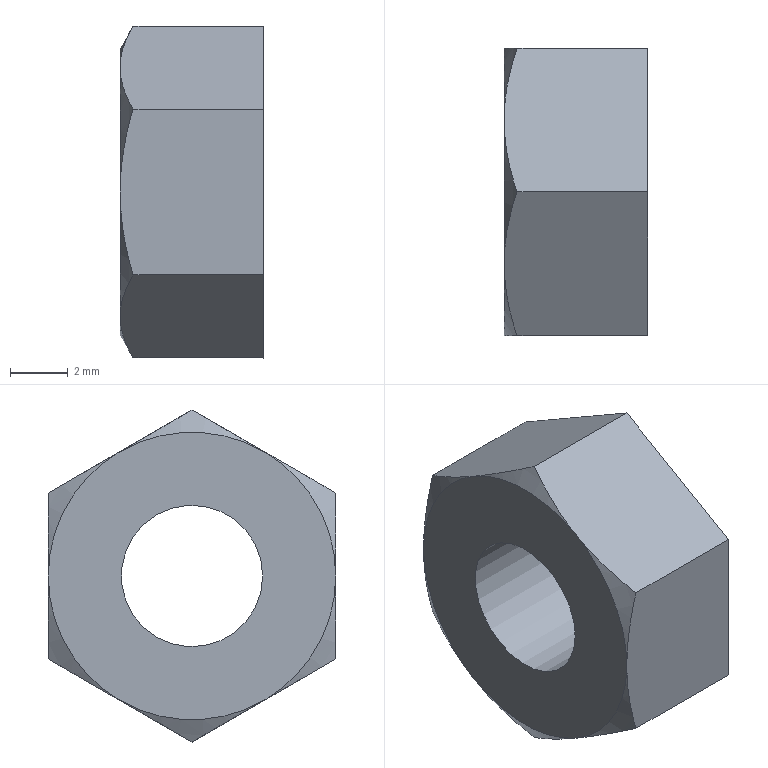Part | NX | features 5003_316_SLBNR6 2 | 1 solid | 15 faces | box 5 x 10 x 11.547 mm | volume 336.962 mm3 | plane 8 | cone 6 | cylinder 1 | commonest cylinder face diameters 4.917 x1
STEP:
#1=CARTESIAN_POINT('',(13.972,-167.,-217.113));
#2=VERTEX_POINT('',#1);
#3=CARTESIAN_POINT('',(18.525,-167.,-217.113));
#4=VERTEX_POINT('',#3);
#5=CARTESIAN_POINT('',(13.525,-167.,-217.113));
#6=DIRECTION('',(1.,0.,0.));
#7=VECTOR('',#6,1000.);
#8=LINE('',#5,#7);
#9=EDGE_CURVE('',#2,#4,#8,.T.);
#10=ORIENTED_EDGE('',*,*,#9,.F.);
#11=CARTESIAN_POINT('',(13.525,-169.5,-215.67));
#12=VERTEX_POINT('',#11);
#13=CARTESIAN_POINT('',(13.972,-167.,-217.113));
#14=CARTESIAN_POINT('',(13.699,-167.818,-216.641));
#15=CARTESIAN_POINT('',(13.525,-168.648,-216.162));
#16=CARTESIAN_POINT('',(13.525,-169.5,-215.67));
#17=B_SPLINE_CURVE_WITH_KNOTS('',3,(#13,#14,#15,#16),.UNSPECIFIED.,.F.,.F.,(4,4),(0.000000238,0.002921),.UNSPECIFIED.);
#18=EDGE_CURVE('',#2,#12,#17,.T.);
#19=ORIENTED_EDGE('',*,*,#18,.T.);
#20=CARTESIAN_POINT('',(13.972,-172.,-214.226));
#21=VERTEX_POINT('',#20);
#22=CARTESIAN_POINT('',(13.525,-169.5,-215.67));
#23=CARTESIAN_POINT('',(13.525,-170.349,-215.18));
#24=CARTESIAN_POINT('',(13.7,-171.184,-214.698));
#25=CARTESIAN_POINT('',(13.972,-172.,-214.226));
#26=B_SPLINE_CURVE_WITH_KNOTS('',3,(#22,#23,#24,#25),.UNSPECIFIED.,.F.,.F.,(4,4),(0.002921,0.005831),.UNSPECIFIED.);
#27=EDGE_CURVE('',#12,#21,#26,.T.);
#28=ORIENTED_EDGE('',*,*,#27,.T.);
#29=CARTESIAN_POINT('',(18.525,-172.,-214.226));
#30=VERTEX_POINT('',#29);
#31=CARTESIAN_POINT('',(13.525,-172.,-214.226));
#32=DIRECTION('',(1.,0.,0.));
#33=VECTOR('',#32,1000.);
#34=LINE('',#31,#33);
#35=EDGE_CURVE('',#21,#30,#34,.T.);
#36=ORIENTED_EDGE('',*,*,#35,.T.);
#37=CARTESIAN_POINT('',(18.525,-167.,-217.113));
#38=DIRECTION('',(0.,-0.866,0.5));
#39=VECTOR('',#38,1000.);
#40=LINE('',#37,#39);
#41=EDGE_CURVE('',#4,#30,#40,.T.);
#42=ORIENTED_EDGE('',*,*,#41,.F.);
#43=EDGE_LOOP('',(#10,#19,#28,#36,#42));
#44=FACE_BOUND('',#43,.T.);
#45=CARTESIAN_POINT('',(13.525,-167.,-217.113));
#46=DIRECTION('',(0.,0.5,0.866));
#47=DIRECTION('',(0.,-0.866,0.5));
#48=AXIS2_PLACEMENT_3D('',#45,#46,#47);
#49=PLANE('',#48);
#50=ADVANCED_FACE('',(#44),#49,.T.);
#51=CARTESIAN_POINT('',(13.972,-167.,-222.887));
#52=VERTEX_POINT('',#51);
#53=CARTESIAN_POINT('',(18.525,-167.,-222.887));
#54=VERTEX_POINT('',#53);
#55=CARTESIAN_POINT('',(13.525,-167.,-222.887));
#56=DIRECTION('',(1.,0.,0.));
#57=VECTOR('',#56,1000.);
#58=LINE('',#55,#57);
#59=EDGE_CURVE('',#52,#54,#58,.T.);
#60=ORIENTED_EDGE('',*,*,#59,.F.);
#61=CARTESIAN_POINT('',(13.525,-167.,-220.));
#62=VERTEX_POINT('',#61);
#63=CARTESIAN_POINT('',(13.972,-167.,-222.887));
#64=CARTESIAN_POINT('',(13.701,-167.,-221.948));
#65=CARTESIAN_POINT('',(13.525,-167.,-220.976));
#66=CARTESIAN_POINT('',(13.525,-167.,-220.));
#67=B_SPLINE_CURVE_WITH_KNOTS('',3,(#63,#64,#65,#66),.UNSPECIFIED.,.F.,.F.,(4,4),(0.00515,0.008071),.UNSPECIFIED.);
#68=EDGE_CURVE('',#52,#62,#67,.T.);
#69=ORIENTED_EDGE('',*,*,#68,.T.);
#70=CARTESIAN_POINT('',(13.525,-167.,-220.));
#71=CARTESIAN_POINT('',(13.525,-167.,-219.024));
#72=CARTESIAN_POINT('',(13.702,-167.,-218.047));
#73=CARTESIAN_POINT('',(13.972,-167.,-217.113));
#74=B_SPLINE_CURVE_WITH_KNOTS('',3,(#70,#71,#72,#73),.UNSPECIFIED.,.F.,.F.,(4,4),(0.008071,0.01099),.UNSPECIFIED.);
#75=EDGE_CURVE('',#62,#2,#74,.T.);
#76=ORIENTED_EDGE('',*,*,#75,.T.);
#77=ORIENTED_EDGE('',*,*,#9,.T.);
#78=CARTESIAN_POINT('',(18.525,-167.,-222.887));
#79=DIRECTION('',(0.,0.,1.));
#80=VECTOR('',#79,1000.);
#81=LINE('',#78,#80);
#82=EDGE_CURVE('',#54,#4,#81,.T.);
#83=ORIENTED_EDGE('',*,*,#82,.F.);
#84=EDGE_LOOP('',(#60,#69,#76,#77,#83));
#85=FACE_BOUND('',#84,.T.);
#86=CARTESIAN_POINT('',(13.525,-167.,-222.887));
#87=DIRECTION('',(0.,1.,0.));
#88=DIRECTION('',(0.,0.,1.));
#89=AXIS2_PLACEMENT_3D('',#86,#87,#88);
#90=PLANE('',#89);
#91=ADVANCED_FACE('',(#85),#90,.T.);
#92=CARTESIAN_POINT('',(13.972,-172.,-225.774));
#93=VERTEX_POINT('',#92);
#94=CARTESIAN_POINT('',(18.525,-172.,-225.774));
#95=VERTEX_POINT('',#94);
#96=CARTESIAN_POINT('',(13.525,-172.,-225.774));
#97=DIRECTION('',(1.,0.,0.));
#98=VECTOR('',#97,1000.);
#99=LINE('',#96,#98);
#100=EDGE_CURVE('',#93,#95,#99,.T.);
#101=ORIENTED_EDGE('',*,*,#100,.F.);
#102=CARTESIAN_POINT('',(13.525,-169.5,-224.33));
#103=VERTEX_POINT('',#102);
#104=CARTESIAN_POINT('',(13.972,-172.,-225.774));
#105=CARTESIAN_POINT('',(13.699,-171.182,-225.301));
#106=CARTESIAN_POINT('',(13.525,-170.352,-224.822));
#107=CARTESIAN_POINT('',(13.525,-169.5,-224.33));
#108=B_SPLINE_CURVE_WITH_KNOTS('',3,(#104,#105,#106,#107),.UNSPECIFIED.,.F.,.F.,(4,4),(0.000000238,0.002921),.UNSPECIFIED.);
#109=EDGE_CURVE('',#93,#103,#108,.T.);
#110=ORIENTED_EDGE('',*,*,#109,.T.);
#111=CARTESIAN_POINT('',(13.525,-169.5,-224.33));
#112=CARTESIAN_POINT('',(13.525,-168.651,-223.84));
#113=CARTESIAN_POINT('',(13.7,-167.816,-223.358));
#114=CARTESIAN_POINT('',(13.972,-167.,-222.887));
#115=B_SPLINE_CURVE_WITH_KNOTS('',3,(#111,#112,#113,#114),.UNSPECIFIED.,.F.,.F.,(4,4),(0.002921,0.005831),.UNSPECIFIED.);
#116=EDGE_CURVE('',#103,#52,#115,.T.);
#117=ORIENTED_EDGE('',*,*,#116,.T.);
#118=ORIENTED_EDGE('',*,*,#59,.T.);
#119=CARTESIAN_POINT('',(18.525,-172.,-225.774));
#120=DIRECTION('',(0.,0.866,0.5));
#121=VECTOR('',#120,1000.);
#122=LINE('',#119,#121);
#123=EDGE_CURVE('',#95,#54,#122,.T.);
#124=ORIENTED_EDGE('',*,*,#123,.F.);
#125=EDGE_LOOP('',(#101,#110,#117,#118,#124));
#126=FACE_BOUND('',#125,.T.);
#127=CARTESIAN_POINT('',(13.525,-172.,-225.774));
#128=DIRECTION('',(0.,0.5,-0.866));
#129=DIRECTION('',(0.,0.866,0.5));
#130=AXIS2_PLACEMENT_3D('',#127,#128,#129);
#131=PLANE('',#130);
#132=ADVANCED_FACE('',(#126),#131,.T.);
#133=CARTESIAN_POINT('',(13.972,-177.,-222.887));
#134=VERTEX_POINT('',#133);
#135=CARTESIAN_POINT('',(18.525,-177.,-222.887));
#136=VERTEX_POINT('',#135);
#137=CARTESIAN_POINT('',(13.525,-177.,-222.887));
#138=DIRECTION('',(1.,0.,0.));
#139=VECTOR('',#138,1000.);
#140=LINE('',#137,#139);
#141=EDGE_CURVE('',#134,#136,#140,.T.);
#142=ORIENTED_EDGE('',*,*,#141,.F.);
#143=CARTESIAN_POINT('',(13.525,-174.5,-224.33));
#144=VERTEX_POINT('',#143);
#145=CARTESIAN_POINT('',(13.972,-177.,-222.887));
#146=CARTESIAN_POINT('',(13.699,-176.182,-223.359));
#147=CARTESIAN_POINT('',(13.525,-175.352,-223.838));
#148=CARTESIAN_POINT('',(13.525,-174.5,-224.33));
#149=B_SPLINE_CURVE_WITH_KNOTS('',3,(#145,#146,#147,#148),.UNSPECIFIED.,.F.,.F.,(4,4),(0.000000238,0.002921),.UNSPECIFIED.);
#150=EDGE_CURVE('',#134,#144,#149,.T.);
#151=ORIENTED_EDGE('',*,*,#150,.T.);
#152=CARTESIAN_POINT('',(13.525,-174.5,-224.33));
#153=CARTESIAN_POINT('',(13.525,-173.651,-224.82));
#154=CARTESIAN_POINT('',(13.7,-172.816,-225.302));
#155=CARTESIAN_POINT('',(13.972,-172.,-225.774));
#156=B_SPLINE_CURVE_WITH_KNOTS('',3,(#152,#153,#154,#155),.UNSPECIFIED.,.F.,.F.,(4,4),(0.002921,0.005831),.UNSPECIFIED.);
#157=EDGE_CURVE('',#144,#93,#156,.T.);
#158=ORIENTED_EDGE('',*,*,#157,.T.);
#159=ORIENTED_EDGE('',*,*,#100,.T.);
#160=CARTESIAN_POINT('',(18.525,-177.,-222.887));
#161=DIRECTION('',(0.,0.866,-0.5));
#162=VECTOR('',#161,1000.);
#163=LINE('',#160,#162);
#164=EDGE_CURVE('',#136,#95,#163,.T.);
#165=ORIENTED_EDGE('',*,*,#164,.F.);
#166=EDGE_LOOP('',(#142,#151,#158,#159,#165));
#167=FACE_BOUND('',#166,.T.);
#168=CARTESIAN_POINT('',(13.525,-177.,-222.887));
#169=DIRECTION('',(0.,-0.5,-0.866));
#170=DIRECTION('',(0.,0.866,-0.5));
#171=AXIS2_PLACEMENT_3D('',#168,#169,#170);
#172=PLANE('',#171);
#173=ADVANCED_FACE('',(#167),#172,.T.);
#174=CARTESIAN_POINT('',(13.972,-177.,-217.113));
#175=VERTEX_POINT('',#174);
#176=CARTESIAN_POINT('',(18.525,-177.,-217.113));
#177=VERTEX_POINT('',#176);
#178=CARTESIAN_POINT('',(13.525,-177.,-217.113));
#179=DIRECTION('',(1.,0.,0.));
#180=VECTOR('',#179,1000.);
#181=LINE('',#178,#180);
#182=EDGE_CURVE('',#175,#177,#181,.T.);
#183=ORIENTED_EDGE('',*,*,#182,.F.);
#184=CARTESIAN_POINT('',(13.525,-177.,-220.));
#185=VERTEX_POINT('',#184);
#186=CARTESIAN_POINT('',(13.525,-177.,-220.));
#187=CARTESIAN_POINT('',(13.525,-177.,-219.024));
#188=CARTESIAN_POINT('',(13.702,-177.,-218.047));
#189=CARTESIAN_POINT('',(13.972,-177.,-217.113));
#190=B_SPLINE_CURVE_WITH_KNOTS('',3,(#186,#187,#188,#189),.UNSPECIFIED.,.F.,.F.,(4,4),(0.008071,0.01099),.UNSPECIFIED.);
#191=EDGE_CURVE('',#175,#185,#190,.F.);
#192=ORIENTED_EDGE('',*,*,#191,.T.);
#193=CARTESIAN_POINT('',(13.972,-177.,-222.887));
#194=CARTESIAN_POINT('',(13.701,-177.,-221.948));
#195=CARTESIAN_POINT('',(13.525,-177.,-220.976));
#196=CARTESIAN_POINT('',(13.525,-177.,-220.));
#197=B_SPLINE_CURVE_WITH_KNOTS('',3,(#193,#194,#195,#196),.UNSPECIFIED.,.F.,.F.,(4,4),(0.00515,0.008071),.UNSPECIFIED.);
#198=EDGE_CURVE('',#185,#134,#197,.F.);
#199=ORIENTED_EDGE('',*,*,#198,.T.);
#200=ORIENTED_EDGE('',*,*,#141,.T.);
#201=CARTESIAN_POINT('',(18.525,-177.,-217.113));
#202=DIRECTION('',(0.,0.,-1.));
#203=VECTOR('',#202,1000.);
#204=LINE('',#201,#203);
#205=EDGE_CURVE('',#177,#136,#204,.T.);
#206=ORIENTED_EDGE('',*,*,#205,.F.);
#207=EDGE_LOOP('',(#183,#192,#199,#200,#206));
#208=FACE_BOUND('',#207,.T.);
#209=CARTESIAN_POINT('',(13.525,-177.,-217.113));
#210=DIRECTION('',(0.,-1.,0.));
#211=DIRECTION('',(0.,0.,-1.));
#212=AXIS2_PLACEMENT_3D('',#209,#210,#211);
#213=PLANE('',#212);
#214=ADVANCED_FACE('',(#208),#213,.T.);
#215=ORIENTED_EDGE('',*,*,#35,.F.);
#216=CARTESIAN_POINT('',(13.525,-174.5,-215.67));
#217=VERTEX_POINT('',#216);
#218=CARTESIAN_POINT('',(13.972,-172.,-214.226));
#219=CARTESIAN_POINT('',(13.699,-172.818,-214.699));
#220=CARTESIAN_POINT('',(13.525,-173.648,-215.178));
#221=CARTESIAN_POINT('',(13.525,-174.5,-215.67));
#222=B_SPLINE_CURVE_WITH_KNOTS('',3,(#218,#219,#220,#221),.UNSPECIFIED.,.F.,.F.,(4,4),(0.000000238,0.002921),.UNSPECIFIED.);
#223=EDGE_CURVE('',#21,#217,#222,.T.);
#224=ORIENTED_EDGE('',*,*,#223,.T.);
#225=CARTESIAN_POINT('',(13.525,-174.5,-215.67));
#226=CARTESIAN_POINT('',(13.525,-175.349,-216.16));
#227=CARTESIAN_POINT('',(13.7,-176.184,-216.642));
#228=CARTESIAN_POINT('',(13.972,-177.,-217.113));
#229=B_SPLINE_CURVE_WITH_KNOTS('',3,(#225,#226,#227,#228),.UNSPECIFIED.,.F.,.F.,(4,4),(0.002921,0.005831),.UNSPECIFIED.);
#230=EDGE_CURVE('',#217,#175,#229,.T.);
#231=ORIENTED_EDGE('',*,*,#230,.T.);
#232=ORIENTED_EDGE('',*,*,#182,.T.);
#233=CARTESIAN_POINT('',(18.525,-172.,-214.226));
#234=DIRECTION('',(0.,-0.866,-0.5));
#235=VECTOR('',#234,1000.);
#236=LINE('',#233,#235);
#237=EDGE_CURVE('',#30,#177,#236,.T.);
#238=ORIENTED_EDGE('',*,*,#237,.F.);
#239=EDGE_LOOP('',(#215,#224,#231,#232,#238));
#240=FACE_BOUND('',#239,.T.);
#241=CARTESIAN_POINT('',(13.525,-172.,-214.226));
#242=DIRECTION('',(0.,-0.5,0.866));
#243=DIRECTION('',(0.,-0.866,-0.5));
#244=AXIS2_PLACEMENT_3D('',#241,#242,#243);
#245=PLANE('',#244);
#246=ADVANCED_FACE('',(#240),#245,.T.);
#247=CARTESIAN_POINT('',(18.525,-174.458,-220.));
#248=VERTEX_POINT('',#247);
#249=CARTESIAN_POINT('',(18.525,-172.,-220.));
#250=DIRECTION('',(-1.,0.,0.));
#251=DIRECTION('',(0.,-1.,0.));
#252=AXIS2_PLACEMENT_3D('',#249,#250,#251);
#253=CIRCLE('',#252,2.458);
#254=EDGE_CURVE('',#248,#248,#253,.T.);
#255=ORIENTED_EDGE('',*,*,#254,.T.);
#256=EDGE_LOOP('',(#255));
#257=FACE_BOUND('',#256,.T.);
#258=ORIENTED_EDGE('',*,*,#41,.T.);
#259=ORIENTED_EDGE('',*,*,#237,.T.);
#260=ORIENTED_EDGE('',*,*,#205,.T.);
#261=ORIENTED_EDGE('',*,*,#164,.T.);
#262=ORIENTED_EDGE('',*,*,#123,.T.);
#263=ORIENTED_EDGE('',*,*,#82,.T.);
#264=EDGE_LOOP('',(#258,#259,#260,#261,#262,#263));
#265=FACE_BOUND('',#264,.T.);
#266=CARTESIAN_POINT('',(18.525,-172.,-220.));
#267=DIRECTION('',(1.,0.,0.));
#268=DIRECTION('',(0.,1.,0.));
#269=AXIS2_PLACEMENT_3D('',#266,#267,#268);
#270=PLANE('',#269);
#271=ADVANCED_FACE('',(#257,#265),#270,.T.);
#272=CARTESIAN_POINT('',(13.525,-172.,-220.));
#273=DIRECTION('',(1.,0.,0.));
#274=DIRECTION('',(0.,1.,0.));
#275=AXIS2_PLACEMENT_3D('',#272,#273,#274);
#276=CIRCLE('',#275,5.);
#277=EDGE_CURVE('',#103,#62,#276,.T.);
#278=ORIENTED_EDGE('',*,*,#277,.T.);
#279=ORIENTED_EDGE('',*,*,#68,.F.);
#280=ORIENTED_EDGE('',*,*,#116,.F.);
#281=EDGE_LOOP('',(#278,#279,#280));
#282=FACE_BOUND('',#281,.T.);
#283=CARTESIAN_POINT('',(13.525,-172.,-220.));
#284=DIRECTION('',(1.,0.,0.));
#285=DIRECTION('',(0.,1.,0.));
#286=AXIS2_PLACEMENT_3D('',#283,#284,#285);
#287=CONICAL_SURFACE('',#286,5.,1.047);
#288=ADVANCED_FACE('',(#282),#287,.T.);
#289=ORIENTED_EDGE('',*,*,#157,.F.);
#290=CARTESIAN_POINT('',(13.525,-172.,-220.));
#291=DIRECTION('',(1.,0.,0.));
#292=DIRECTION('',(0.,1.,0.));
#293=AXIS2_PLACEMENT_3D('',#290,#291,#292);
#294=CIRCLE('',#293,5.);
#295=EDGE_CURVE('',#144,#103,#294,.T.);
#296=ORIENTED_EDGE('',*,*,#295,.T.);
#297=ORIENTED_EDGE('',*,*,#109,.F.);
#298=EDGE_LOOP('',(#289,#296,#297));
#299=FACE_BOUND('',#298,.T.);
#300=CARTESIAN_POINT('',(13.525,-172.,-220.));
#301=DIRECTION('',(1.,0.,0.));
#302=DIRECTION('',(0.,1.,0.));
#303=AXIS2_PLACEMENT_3D('',#300,#301,#302);
#304=CONICAL_SURFACE('',#303,5.,1.047);
#305=ADVANCED_FACE('',(#299),#304,.T.);
#306=ORIENTED_EDGE('',*,*,#198,.F.);
#307=CARTESIAN_POINT('',(13.525,-172.,-220.));
#308=DIRECTION('',(1.,0.,0.));
#309=DIRECTION('',(0.,1.,0.));
#310=AXIS2_PLACEMENT_3D('',#307,#308,#309);
#311=CIRCLE('',#310,5.);
#312=EDGE_CURVE('',#185,#144,#311,.T.);
#313=ORIENTED_EDGE('',*,*,#312,.T.);
#314=ORIENTED_EDGE('',*,*,#150,.F.);
#315=EDGE_LOOP('',(#306,#313,#314));
#316=FACE_BOUND('',#315,.T.);
#317=CARTESIAN_POINT('',(13.525,-172.,-220.));
#318=DIRECTION('',(1.,0.,0.));
#319=DIRECTION('',(0.,1.,0.));
#320=AXIS2_PLACEMENT_3D('',#317,#318,#319);
#321=CONICAL_SURFACE('',#320,5.,1.047);
#322=ADVANCED_FACE('',(#316),#321,.T.);
#323=ORIENTED_EDGE('',*,*,#230,.F.);
#324=CARTESIAN_POINT('',(13.525,-172.,-220.));
#325=DIRECTION('',(-1.,0.,0.));
#326=DIRECTION('',(0.,-1.,0.));
#327=AXIS2_PLACEMENT_3D('',#324,#325,#326);
#328=CIRCLE('',#327,5.);
#329=EDGE_CURVE('',#185,#217,#328,.T.);
#330=ORIENTED_EDGE('',*,*,#329,.F.);
#331=ORIENTED_EDGE('',*,*,#191,.F.);
#332=EDGE_LOOP('',(#323,#330,#331));
#333=FACE_BOUND('',#332,.T.);
#334=CARTESIAN_POINT('',(13.525,-172.,-220.));
#335=DIRECTION('',(1.,0.,0.));
#336=DIRECTION('',(0.,1.,0.));
#337=AXIS2_PLACEMENT_3D('',#334,#335,#336);
#338=CONICAL_SURFACE('',#337,5.,1.047);
#339=ADVANCED_FACE('',(#333),#338,.T.);
#340=CARTESIAN_POINT('',(13.525,-172.,-220.));
#341=DIRECTION('',(1.,0.,0.));
#342=DIRECTION('',(0.,1.,0.));
#343=AXIS2_PLACEMENT_3D('',#340,#341,#342);
#344=CIRCLE('',#343,5.);
#345=EDGE_CURVE('',#12,#217,#344,.T.);
#346=ORIENTED_EDGE('',*,*,#345,.T.);
#347=ORIENTED_EDGE('',*,*,#223,.F.);
#348=ORIENTED_EDGE('',*,*,#27,.F.);
#349=EDGE_LOOP('',(#346,#347,#348));
#350=FACE_BOUND('',#349,.T.);
#351=CARTESIAN_POINT('',(13.525,-172.,-220.));
#352=DIRECTION('',(1.,0.,0.));
#353=DIRECTION('',(0.,1.,0.));
#354=AXIS2_PLACEMENT_3D('',#351,#352,#353);
#355=CONICAL_SURFACE('',#354,5.,1.047);
#356=ADVANCED_FACE('',(#350),#355,.T.);
#357=CARTESIAN_POINT('',(13.525,-172.,-220.));
#358=DIRECTION('',(1.,0.,0.));
#359=DIRECTION('',(0.,1.,0.));
#360=AXIS2_PLACEMENT_3D('',#357,#358,#359);
#361=CIRCLE('',#360,5.);
#362=EDGE_CURVE('',#62,#12,#361,.T.);
#363=ORIENTED_EDGE('',*,*,#362,.T.);
#364=ORIENTED_EDGE('',*,*,#18,.F.);
#365=ORIENTED_EDGE('',*,*,#75,.F.);
#366=EDGE_LOOP('',(#363,#364,#365));
#367=FACE_BOUND('',#366,.T.);
#368=CARTESIAN_POINT('',(13.525,-172.,-220.));
#369=DIRECTION('',(1.,0.,0.));
#370=DIRECTION('',(0.,1.,0.));
#371=AXIS2_PLACEMENT_3D('',#368,#369,#370);
#372=CONICAL_SURFACE('',#371,5.,1.047);
#373=ADVANCED_FACE('',(#367),#372,.T.);
#374=CARTESIAN_POINT('',(13.525,-174.458,-220.));
#375=VERTEX_POINT('',#374);
#376=CARTESIAN_POINT('',(13.525,-172.,-220.));
#377=DIRECTION('',(-1.,0.,0.));
#378=DIRECTION('',(0.,-1.,0.));
#379=AXIS2_PLACEMENT_3D('',#376,#377,#378);
#380=CIRCLE('',#379,2.458);
#381=EDGE_CURVE('',#375,#375,#380,.T.);
#382=ORIENTED_EDGE('',*,*,#381,.F.);
#383=EDGE_LOOP('',(#382));
#384=FACE_BOUND('',#383,.T.);
#385=ORIENTED_EDGE('',*,*,#362,.F.);
#386=ORIENTED_EDGE('',*,*,#277,.F.);
#387=ORIENTED_EDGE('',*,*,#295,.F.);
#388=ORIENTED_EDGE('',*,*,#312,.F.);
#389=ORIENTED_EDGE('',*,*,#329,.T.);
#390=ORIENTED_EDGE('',*,*,#345,.F.);
#391=EDGE_LOOP('',(#385,#386,#387,#388,#389,#390));
#392=FACE_BOUND('',#391,.T.);
#393=CARTESIAN_POINT('',(13.525,-172.,-220.));
#394=DIRECTION('',(1.,0.,0.));
#395=DIRECTION('',(0.,1.,0.));
#396=AXIS2_PLACEMENT_3D('',#393,#394,#395);
#397=PLANE('',#396);
#398=ADVANCED_FACE('',(#384,#392),#397,.F.);
#399=ORIENTED_EDGE('',*,*,#254,.F.);
#400=EDGE_LOOP('',(#399));
#401=FACE_BOUND('',#400,.T.);
#402=ORIENTED_EDGE('',*,*,#381,.T.);
#403=EDGE_LOOP('',(#402));
#404=FACE_BOUND('',#403,.T.);
#405=CARTESIAN_POINT('',(13.525,-172.,-220.));
#406=DIRECTION('',(-1.,0.,0.));
#407=DIRECTION('',(0.,-1.,0.));
#408=AXIS2_PLACEMENT_3D('',#405,#406,#407);
#409=CYLINDRICAL_SURFACE('',#408,2.458);
#410=ADVANCED_FACE('',(#401,#404),#409,.F.);
#411=CLOSED_SHELL('',(#50,#91,#132,#173,#214,#246,#271,#288,#305,#322,#339,#356,#373,#398,#410));
#412=MANIFOLD_SOLID_BREP('',#411);
#413=(LENGTH_UNIT()NAMED_UNIT(*)SI_UNIT(.MILLI.,.METRE.));
#414=UNCERTAINTY_MEASURE_WITH_UNIT(LENGTH_MEASURE(0.0508),#413,'','');
#415=(NAMED_UNIT(*)PLANE_ANGLE_UNIT()SI_UNIT($,.RADIAN.));
#416=(NAMED_UNIT(*)SI_UNIT($,.STERADIAN.)SOLID_ANGLE_UNIT());
#417=(GEOMETRIC_REPRESENTATION_CONTEXT(3)GLOBAL_UNCERTAINTY_ASSIGNED_CONTEXT((#414))GLOBAL_UNIT_ASSIGNED_CONTEXT((#413,#415,#416))REPRESENTATION_CONTEXT('',''));
#418=ADVANCED_BREP_SHAPE_REPRESENTATION('',(#412),#417);